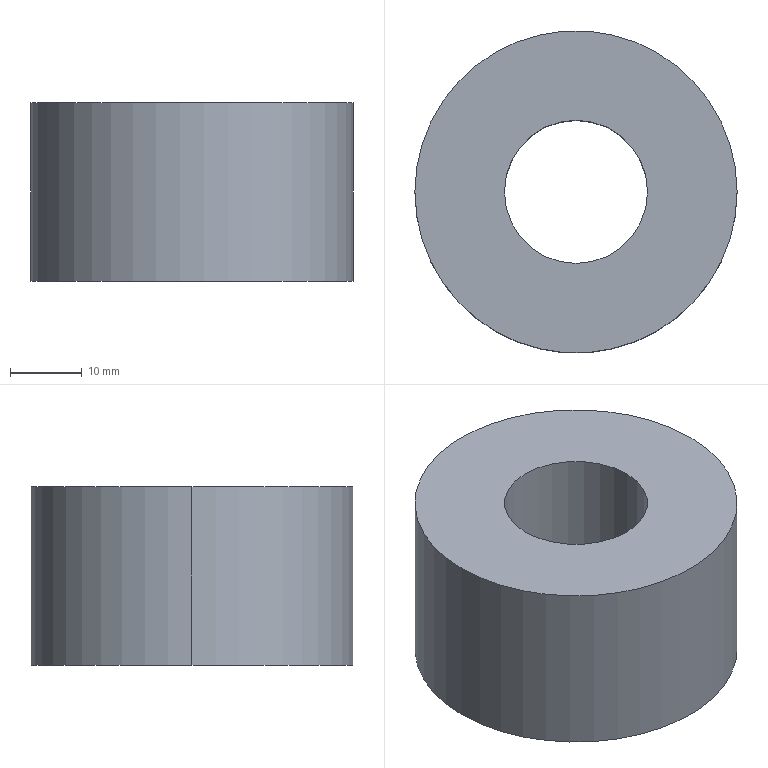Part | STEP file | BU-A02b | 1 solid | 6 faces | box 45 x 45 x 25 mm | volume 31907 mm3 | cylinder 4 | plane 2 | commonest cylinder face diameters 20 x2 45 x2
STEP:
#1=CARTESIAN_POINT('',(0.,0.,0.));
#2=DIRECTION('',(0.,0.,1.));
#3=DIRECTION('',(1.,0.,0.));
#4=AXIS2_PLACEMENT_3D('',#1,#2,#3);
#5=CARTESIAN_POINT('',(-10.,0.,25.));
#6=VERTEX_POINT('',#5);
#7=CARTESIAN_POINT('',(-10.,0.,0.));
#8=VERTEX_POINT('',#7);
#9=CARTESIAN_POINT('',(-10.,0.,25.));
#10=DIRECTION('',(0.,0.,-1.));
#11=VECTOR('',#10,1.);
#12=LINE('',#9,#11);
#13=CARTESIAN_POINT('',(0.,0.,25.));
#14=DIRECTION('',(0.,0.,-1.));
#15=DIRECTION('',(-1.,0.,0.));
#16=AXIS2_PLACEMENT_3D('',#13,#14,#15);
#17=CYLINDRICAL_SURFACE('',#16,10.);
#18=CARTESIAN_POINT('',(6.283,0.));
#19=DIRECTION('',(0.,1.));
#20=VECTOR('',#19,1.);
#21=LINE('',#18,#20);
#22=(GEOMETRIC_REPRESENTATION_CONTEXT(2)PARAMETRIC_REPRESENTATION_CONTEXT()REPRESENTATION_CONTEXT('',''));
#23=DEFINITIONAL_REPRESENTATION('',(#21),#22);
#24=PCURVE('',#17,#23);
#25=CARTESIAN_POINT('',(0.,0.,25.));
#26=DIRECTION('',(0.,0.,-1.));
#27=DIRECTION('',(-1.,0.,0.));
#28=AXIS2_PLACEMENT_3D('',#25,#26,#27);
#29=CYLINDRICAL_SURFACE('',#28,10.);
#30=CARTESIAN_POINT('',(0.,0.));
#31=DIRECTION('',(0.,1.));
#32=VECTOR('',#31,1.);
#33=LINE('',#30,#32);
#34=(GEOMETRIC_REPRESENTATION_CONTEXT(2)PARAMETRIC_REPRESENTATION_CONTEXT()REPRESENTATION_CONTEXT('',''));
#35=DEFINITIONAL_REPRESENTATION('',(#33),#34);
#36=PCURVE('',#29,#35);
#37=SURFACE_CURVE('',#12,(#24,#36),.PCURVE_S1.);
#38=EDGE_CURVE('',#6,#8,#37,.T.);
#39=ORIENTED_EDGE('',*,*,#38,.T.);
#40=CARTESIAN_POINT('',(10.,0.,0.));
#41=VERTEX_POINT('',#40);
#42=CARTESIAN_POINT('',(0.,0.,0.));
#43=DIRECTION('',(0.,0.,1.));
#44=DIRECTION('',(1.,0.,0.));
#45=AXIS2_PLACEMENT_3D('',#42,#43,#44);
#46=CIRCLE('',#45,10.);
#47=CARTESIAN_POINT('',(9.425,25.));
#48=DIRECTION('',(-1.,0.));
#49=VECTOR('',#48,1.);
#50=LINE('',#47,#49);
#51=(GEOMETRIC_REPRESENTATION_CONTEXT(2)PARAMETRIC_REPRESENTATION_CONTEXT()REPRESENTATION_CONTEXT('',''));
#52=DEFINITIONAL_REPRESENTATION('',(#50),#51);
#53=PCURVE('',#17,#52);
#54=CARTESIAN_POINT('',(0.,0.,0.));
#55=DIRECTION('',(0.,0.,1.));
#56=DIRECTION('',(1.,0.,0.));
#57=AXIS2_PLACEMENT_3D('',#54,#55,#56);
#58=PLANE('',#57);
#59=CARTESIAN_POINT('',(0.,0.));
#60=DIRECTION('',(1.,0.));
#61=AXIS2_PLACEMENT_2D('',#59,#60);
#62=CIRCLE('',#61,10.);
#63=(GEOMETRIC_REPRESENTATION_CONTEXT(2)PARAMETRIC_REPRESENTATION_CONTEXT()REPRESENTATION_CONTEXT('',''));
#64=DEFINITIONAL_REPRESENTATION('',(#62),#63);
#65=PCURVE('',#58,#64);
#66=SURFACE_CURVE('',#46,(#53,#65),.PCURVE_S1.);
#67=EDGE_CURVE('',#8,#41,#66,.T.);
#68=ORIENTED_EDGE('',*,*,#67,.T.);
#69=CARTESIAN_POINT('',(10.,0.,25.));
#70=VERTEX_POINT('',#69);
#71=CARTESIAN_POINT('',(10.,0.,25.));
#72=DIRECTION('',(0.,0.,-1.));
#73=VECTOR('',#72,1.);
#74=LINE('',#71,#73);
#75=CARTESIAN_POINT('',(3.142,0.));
#76=DIRECTION('',(0.,1.));
#77=VECTOR('',#76,1.);
#78=LINE('',#75,#77);
#79=(GEOMETRIC_REPRESENTATION_CONTEXT(2)PARAMETRIC_REPRESENTATION_CONTEXT()REPRESENTATION_CONTEXT('',''));
#80=DEFINITIONAL_REPRESENTATION('',(#78),#79);
#81=PCURVE('',#17,#80);
#82=CARTESIAN_POINT('',(3.142,0.));
#83=DIRECTION('',(0.,1.));
#84=VECTOR('',#83,1.);
#85=LINE('',#82,#84);
#86=(GEOMETRIC_REPRESENTATION_CONTEXT(2)PARAMETRIC_REPRESENTATION_CONTEXT()REPRESENTATION_CONTEXT('',''));
#87=DEFINITIONAL_REPRESENTATION('',(#85),#86);
#88=PCURVE('',#29,#87);
#89=SURFACE_CURVE('',#74,(#81,#88),.PCURVE_S1.);
#90=EDGE_CURVE('',#70,#41,#89,.T.);
#91=ORIENTED_EDGE('',*,*,#90,.F.);
#92=CARTESIAN_POINT('',(0.,0.,25.));
#93=DIRECTION('',(0.,0.,1.));
#94=DIRECTION('',(1.,0.,0.));
#95=AXIS2_PLACEMENT_3D('',#92,#93,#94);
#96=CIRCLE('',#95,10.);
#97=CARTESIAN_POINT('',(9.425,0.));
#98=DIRECTION('',(-1.,0.));
#99=VECTOR('',#98,1.);
#100=LINE('',#97,#99);
#101=(GEOMETRIC_REPRESENTATION_CONTEXT(2)PARAMETRIC_REPRESENTATION_CONTEXT()REPRESENTATION_CONTEXT('',''));
#102=DEFINITIONAL_REPRESENTATION('',(#100),#101);
#103=PCURVE('',#17,#102);
#104=CARTESIAN_POINT('',(0.,0.,25.));
#105=DIRECTION('',(0.,0.,1.));
#106=DIRECTION('',(1.,0.,0.));
#107=AXIS2_PLACEMENT_3D('',#104,#105,#106);
#108=PLANE('',#107);
#109=CARTESIAN_POINT('',(0.,0.));
#110=DIRECTION('',(1.,0.));
#111=AXIS2_PLACEMENT_2D('',#109,#110);
#112=CIRCLE('',#111,10.);
#113=(GEOMETRIC_REPRESENTATION_CONTEXT(2)PARAMETRIC_REPRESENTATION_CONTEXT()REPRESENTATION_CONTEXT('',''));
#114=DEFINITIONAL_REPRESENTATION('',(#112),#113);
#115=PCURVE('',#108,#114);
#116=SURFACE_CURVE('',#96,(#103,#115),.PCURVE_S1.);
#117=EDGE_CURVE('',#6,#70,#116,.T.);
#118=ORIENTED_EDGE('',*,*,#117,.F.);
#119=EDGE_LOOP('',(#39,#68,#91,#118));
#120=FACE_BOUND('',#119,.F.);
#121=ADVANCED_FACE('',(#120),#17,.F.);
#122=CARTESIAN_POINT('',(22.5,0.,25.));
#123=VERTEX_POINT('',#122);
#124=CARTESIAN_POINT('',(-22.5,0.,25.));
#125=VERTEX_POINT('',#124);
#126=CARTESIAN_POINT('',(0.,0.,25.));
#127=DIRECTION('',(0.,0.,1.));
#128=DIRECTION('',(1.,0.,0.));
#129=AXIS2_PLACEMENT_3D('',#126,#127,#128);
#130=CIRCLE('',#129,22.5);
#131=CARTESIAN_POINT('',(0.,0.,25.));
#132=DIRECTION('',(0.,0.,-1.));
#133=DIRECTION('',(-1.,0.,0.));
#134=AXIS2_PLACEMENT_3D('',#131,#132,#133);
#135=CYLINDRICAL_SURFACE('',#134,22.5);
#136=CARTESIAN_POINT('',(3.142,0.));
#137=DIRECTION('',(-1.,0.));
#138=VECTOR('',#137,1.);
#139=LINE('',#136,#138);
#140=(GEOMETRIC_REPRESENTATION_CONTEXT(2)PARAMETRIC_REPRESENTATION_CONTEXT()REPRESENTATION_CONTEXT('',''));
#141=DEFINITIONAL_REPRESENTATION('',(#139),#140);
#142=PCURVE('',#135,#141);
#143=CARTESIAN_POINT('',(0.,0.));
#144=DIRECTION('',(1.,0.));
#145=AXIS2_PLACEMENT_2D('',#143,#144);
#146=CIRCLE('',#145,22.5);
#147=(GEOMETRIC_REPRESENTATION_CONTEXT(2)PARAMETRIC_REPRESENTATION_CONTEXT()REPRESENTATION_CONTEXT('',''));
#148=DEFINITIONAL_REPRESENTATION('',(#146),#147);
#149=PCURVE('',#108,#148);
#150=SURFACE_CURVE('',#130,(#142,#149),.PCURVE_S1.);
#151=EDGE_CURVE('',#123,#125,#150,.T.);
#152=ORIENTED_EDGE('',*,*,#151,.F.);
#153=CARTESIAN_POINT('',(22.5,0.,0.));
#154=VERTEX_POINT('',#153);
#155=CARTESIAN_POINT('',(22.5,0.,25.));
#156=DIRECTION('',(0.,0.,-1.));
#157=VECTOR('',#156,1.);
#158=LINE('',#155,#157);
#159=CARTESIAN_POINT('',(3.142,0.));
#160=DIRECTION('',(0.,1.));
#161=VECTOR('',#160,1.);
#162=LINE('',#159,#161);
#163=(GEOMETRIC_REPRESENTATION_CONTEXT(2)PARAMETRIC_REPRESENTATION_CONTEXT()REPRESENTATION_CONTEXT('',''));
#164=DEFINITIONAL_REPRESENTATION('',(#162),#163);
#165=PCURVE('',#135,#164);
#166=CARTESIAN_POINT('',(0.,0.,25.));
#167=DIRECTION('',(0.,0.,-1.));
#168=DIRECTION('',(-1.,0.,0.));
#169=AXIS2_PLACEMENT_3D('',#166,#167,#168);
#170=CYLINDRICAL_SURFACE('',#169,22.5);
#171=CARTESIAN_POINT('',(3.142,0.));
#172=DIRECTION('',(0.,1.));
#173=VECTOR('',#172,1.);
#174=LINE('',#171,#173);
#175=(GEOMETRIC_REPRESENTATION_CONTEXT(2)PARAMETRIC_REPRESENTATION_CONTEXT()REPRESENTATION_CONTEXT('',''));
#176=DEFINITIONAL_REPRESENTATION('',(#174),#175);
#177=PCURVE('',#170,#176);
#178=SURFACE_CURVE('',#158,(#165,#177),.PCURVE_S1.);
#179=EDGE_CURVE('',#123,#154,#178,.T.);
#180=ORIENTED_EDGE('',*,*,#179,.T.);
#181=CARTESIAN_POINT('',(-22.5,0.,0.));
#182=VERTEX_POINT('',#181);
#183=CARTESIAN_POINT('',(0.,0.,0.));
#184=DIRECTION('',(0.,0.,1.));
#185=DIRECTION('',(1.,0.,0.));
#186=AXIS2_PLACEMENT_3D('',#183,#184,#185);
#187=CIRCLE('',#186,22.5);
#188=CARTESIAN_POINT('',(3.142,25.));
#189=DIRECTION('',(-1.,0.));
#190=VECTOR('',#189,1.);
#191=LINE('',#188,#190);
#192=(GEOMETRIC_REPRESENTATION_CONTEXT(2)PARAMETRIC_REPRESENTATION_CONTEXT()REPRESENTATION_CONTEXT('',''));
#193=DEFINITIONAL_REPRESENTATION('',(#191),#192);
#194=PCURVE('',#135,#193);
#195=CARTESIAN_POINT('',(0.,0.));
#196=DIRECTION('',(1.,0.));
#197=AXIS2_PLACEMENT_2D('',#195,#196);
#198=CIRCLE('',#197,22.5);
#199=(GEOMETRIC_REPRESENTATION_CONTEXT(2)PARAMETRIC_REPRESENTATION_CONTEXT()REPRESENTATION_CONTEXT('',''));
#200=DEFINITIONAL_REPRESENTATION('',(#198),#199);
#201=PCURVE('',#58,#200);
#202=SURFACE_CURVE('',#187,(#194,#201),.PCURVE_S1.);
#203=EDGE_CURVE('',#154,#182,#202,.T.);
#204=ORIENTED_EDGE('',*,*,#203,.T.);
#205=CARTESIAN_POINT('',(-22.5,0.,25.));
#206=DIRECTION('',(0.,0.,-1.));
#207=VECTOR('',#206,1.);
#208=LINE('',#205,#207);
#209=CARTESIAN_POINT('',(0.,0.));
#210=DIRECTION('',(0.,1.));
#211=VECTOR('',#210,1.);
#212=LINE('',#209,#211);
#213=(GEOMETRIC_REPRESENTATION_CONTEXT(2)PARAMETRIC_REPRESENTATION_CONTEXT()REPRESENTATION_CONTEXT('',''));
#214=DEFINITIONAL_REPRESENTATION('',(#212),#213);
#215=PCURVE('',#135,#214);
#216=CARTESIAN_POINT('',(6.283,0.));
#217=DIRECTION('',(0.,1.));
#218=VECTOR('',#217,1.);
#219=LINE('',#216,#218);
#220=(GEOMETRIC_REPRESENTATION_CONTEXT(2)PARAMETRIC_REPRESENTATION_CONTEXT()REPRESENTATION_CONTEXT('',''));
#221=DEFINITIONAL_REPRESENTATION('',(#219),#220);
#222=PCURVE('',#170,#221);
#223=SURFACE_CURVE('',#208,(#215,#222),.PCURVE_S1.);
#224=EDGE_CURVE('',#125,#182,#223,.T.);
#225=ORIENTED_EDGE('',*,*,#224,.F.);
#226=EDGE_LOOP('',(#152,#180,#204,#225));
#227=FACE_BOUND('',#226,.T.);
#228=ADVANCED_FACE('',(#227),#135,.T.);
#229=CARTESIAN_POINT('',(0.,0.,25.));
#230=DIRECTION('',(0.,0.,1.));
#231=DIRECTION('',(1.,0.,0.));
#232=AXIS2_PLACEMENT_3D('',#229,#230,#231);
#233=CIRCLE('',#232,22.5);
#234=CARTESIAN_POINT('',(0.,0.));
#235=DIRECTION('',(1.,0.));
#236=AXIS2_PLACEMENT_2D('',#234,#235);
#237=CIRCLE('',#236,22.5);
#238=(GEOMETRIC_REPRESENTATION_CONTEXT(2)PARAMETRIC_REPRESENTATION_CONTEXT()REPRESENTATION_CONTEXT('',''));
#239=DEFINITIONAL_REPRESENTATION('',(#237),#238);
#240=PCURVE('',#108,#239);
#241=CARTESIAN_POINT('',(9.425,0.));
#242=DIRECTION('',(-1.,0.));
#243=VECTOR('',#242,1.);
#244=LINE('',#241,#243);
#245=(GEOMETRIC_REPRESENTATION_CONTEXT(2)PARAMETRIC_REPRESENTATION_CONTEXT()REPRESENTATION_CONTEXT('',''));
#246=DEFINITIONAL_REPRESENTATION('',(#244),#245);
#247=PCURVE('',#170,#246);
#248=SURFACE_CURVE('',#233,(#240,#247),.PCURVE_S1.);
#249=EDGE_CURVE('',#125,#123,#248,.T.);
#250=ORIENTED_EDGE('',*,*,#249,.T.);
#251=ORIENTED_EDGE('',*,*,#151,.T.);
#252=EDGE_LOOP('',(#250,#251));
#253=FACE_BOUND('',#252,.T.);
#254=ORIENTED_EDGE('',*,*,#117,.F.);
#255=CARTESIAN_POINT('',(0.,0.,25.));
#256=DIRECTION('',(0.,0.,1.));
#257=DIRECTION('',(1.,0.,0.));
#258=AXIS2_PLACEMENT_3D('',#255,#256,#257);
#259=CIRCLE('',#258,10.);
#260=CARTESIAN_POINT('',(0.,0.));
#261=DIRECTION('',(1.,0.));
#262=AXIS2_PLACEMENT_2D('',#260,#261);
#263=CIRCLE('',#262,10.);
#264=(GEOMETRIC_REPRESENTATION_CONTEXT(2)PARAMETRIC_REPRESENTATION_CONTEXT()REPRESENTATION_CONTEXT('',''));
#265=DEFINITIONAL_REPRESENTATION('',(#263),#264);
#266=PCURVE('',#108,#265);
#267=CARTESIAN_POINT('',(3.142,0.));
#268=DIRECTION('',(-1.,0.));
#269=VECTOR('',#268,1.);
#270=LINE('',#267,#269);
#271=(GEOMETRIC_REPRESENTATION_CONTEXT(2)PARAMETRIC_REPRESENTATION_CONTEXT()REPRESENTATION_CONTEXT('',''));
#272=DEFINITIONAL_REPRESENTATION('',(#270),#271);
#273=PCURVE('',#29,#272);
#274=SURFACE_CURVE('',#259,(#266,#273),.PCURVE_S1.);
#275=EDGE_CURVE('',#70,#6,#274,.T.);
#276=ORIENTED_EDGE('',*,*,#275,.F.);
#277=EDGE_LOOP('',(#254,#276));
#278=FACE_BOUND('',#277,.T.);
#279=ADVANCED_FACE('',(#253,#278),#108,.T.);
#280=CARTESIAN_POINT('',(0.,0.,0.));
#281=DIRECTION('',(0.,0.,1.));
#282=DIRECTION('',(1.,0.,0.));
#283=AXIS2_PLACEMENT_3D('',#280,#281,#282);
#284=CIRCLE('',#283,22.5);
#285=CARTESIAN_POINT('',(0.,0.));
#286=DIRECTION('',(1.,0.));
#287=AXIS2_PLACEMENT_2D('',#285,#286);
#288=CIRCLE('',#287,22.5);
#289=(GEOMETRIC_REPRESENTATION_CONTEXT(2)PARAMETRIC_REPRESENTATION_CONTEXT()REPRESENTATION_CONTEXT('',''));
#290=DEFINITIONAL_REPRESENTATION('',(#288),#289);
#291=PCURVE('',#58,#290);
#292=CARTESIAN_POINT('',(9.425,25.));
#293=DIRECTION('',(-1.,0.));
#294=VECTOR('',#293,1.);
#295=LINE('',#292,#294);
#296=(GEOMETRIC_REPRESENTATION_CONTEXT(2)PARAMETRIC_REPRESENTATION_CONTEXT()REPRESENTATION_CONTEXT('',''));
#297=DEFINITIONAL_REPRESENTATION('',(#295),#296);
#298=PCURVE('',#170,#297);
#299=SURFACE_CURVE('',#284,(#291,#298),.PCURVE_S1.);
#300=EDGE_CURVE('',#182,#154,#299,.T.);
#301=ORIENTED_EDGE('',*,*,#300,.F.);
#302=ORIENTED_EDGE('',*,*,#203,.F.);
#303=EDGE_LOOP('',(#301,#302));
#304=FACE_BOUND('',#303,.T.);
#305=ORIENTED_EDGE('',*,*,#67,.T.);
#306=CARTESIAN_POINT('',(0.,0.,0.));
#307=DIRECTION('',(0.,0.,1.));
#308=DIRECTION('',(1.,0.,0.));
#309=AXIS2_PLACEMENT_3D('',#306,#307,#308);
#310=CIRCLE('',#309,10.);
#311=CARTESIAN_POINT('',(0.,0.));
#312=DIRECTION('',(1.,0.));
#313=AXIS2_PLACEMENT_2D('',#311,#312);
#314=CIRCLE('',#313,10.);
#315=(GEOMETRIC_REPRESENTATION_CONTEXT(2)PARAMETRIC_REPRESENTATION_CONTEXT()REPRESENTATION_CONTEXT('',''));
#316=DEFINITIONAL_REPRESENTATION('',(#314),#315);
#317=PCURVE('',#58,#316);
#318=CARTESIAN_POINT('',(3.142,25.));
#319=DIRECTION('',(-1.,0.));
#320=VECTOR('',#319,1.);
#321=LINE('',#318,#320);
#322=(GEOMETRIC_REPRESENTATION_CONTEXT(2)PARAMETRIC_REPRESENTATION_CONTEXT()REPRESENTATION_CONTEXT('',''));
#323=DEFINITIONAL_REPRESENTATION('',(#321),#322);
#324=PCURVE('',#29,#323);
#325=SURFACE_CURVE('',#310,(#317,#324),.PCURVE_S1.);
#326=EDGE_CURVE('',#41,#8,#325,.T.);
#327=ORIENTED_EDGE('',*,*,#326,.T.);
#328=EDGE_LOOP('',(#305,#327));
#329=FACE_BOUND('',#328,.T.);
#330=ADVANCED_FACE('',(#304,#329),#58,.F.);
#331=ORIENTED_EDGE('',*,*,#179,.F.);
#332=ORIENTED_EDGE('',*,*,#249,.F.);
#333=ORIENTED_EDGE('',*,*,#224,.T.);
#334=ORIENTED_EDGE('',*,*,#300,.T.);
#335=EDGE_LOOP('',(#331,#332,#333,#334));
#336=FACE_BOUND('',#335,.T.);
#337=ADVANCED_FACE('',(#336),#170,.T.);
#338=ORIENTED_EDGE('',*,*,#326,.T.);
#339=ORIENTED_EDGE('',*,*,#38,.F.);
#340=ORIENTED_EDGE('',*,*,#275,.F.);
#341=ORIENTED_EDGE('',*,*,#90,.T.);
#342=EDGE_LOOP('',(#338,#339,#340,#341));
#343=FACE_BOUND('',#342,.F.);
#344=ADVANCED_FACE('',(#343),#29,.F.);
#345=CLOSED_SHELL('',(#121,#228,#279,#330,#337,#344));
#346=MANIFOLD_SOLID_BREP('',#345);
#347=(LENGTH_UNIT()NAMED_UNIT(*)SI_UNIT(.MILLI.,.METRE.));
#348=UNCERTAINTY_MEASURE_WITH_UNIT(LENGTH_MEASURE(0.0000001),#347,'','');
#349=(NAMED_UNIT(*)PLANE_ANGLE_UNIT()SI_UNIT($,.RADIAN.));
#350=(NAMED_UNIT(*)SI_UNIT($,.STERADIAN.)SOLID_ANGLE_UNIT());
#351=(GEOMETRIC_REPRESENTATION_CONTEXT(3)GLOBAL_UNCERTAINTY_ASSIGNED_CONTEXT((#348))GLOBAL_UNIT_ASSIGNED_CONTEXT((#347,#349,#350))REPRESENTATION_CONTEXT('',''));
#352=ADVANCED_BREP_SHAPE_REPRESENTATION('',(#4,#346),#351);